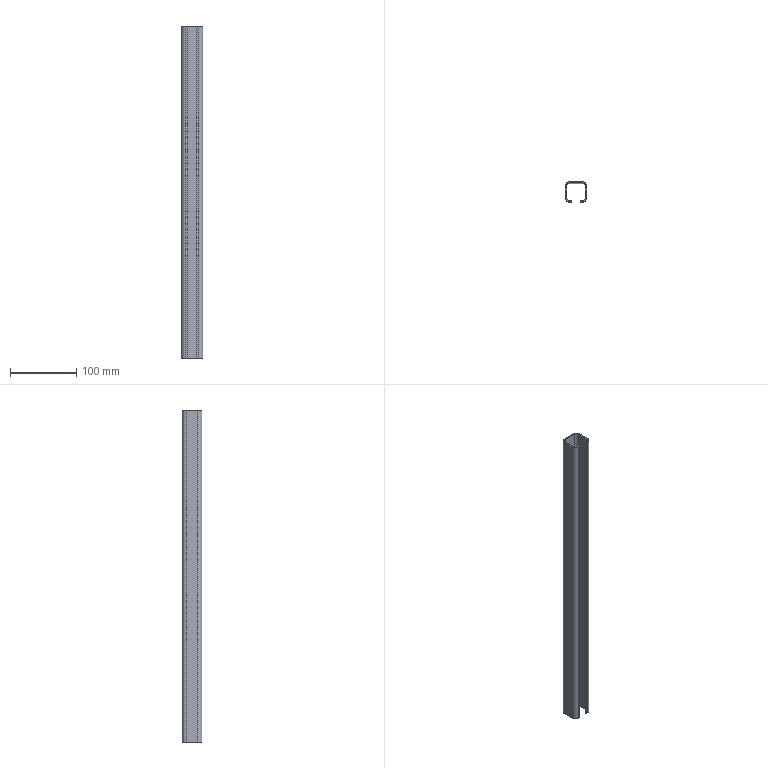Part | SolidWorks | features Extrusion 1 | 1 solid | 22 faces | box 32 x 30 x 500 mm | volume 85540 mm3 | plane 14 | cylinder 8 | commonest cylinder face diameters 8.4 x4 12 x4
STEP:
#1=CARTESIAN_POINT('',(-16.,-9.,0.));
#2=VERTEX_POINT('',#1);
#3=CARTESIAN_POINT('',(-10.,-15.,0.));
#4=VERTEX_POINT('',#3);
#5=CARTESIAN_POINT('',(-10.,-9.,0.));
#6=DIRECTION('',(0.,0.,1.));
#7=DIRECTION('',(1.,0.,0.));
#8=AXIS2_PLACEMENT_3D('',#5,#6,#7);
#9=CIRCLE('',#8,6.);
#10=EDGE_CURVE('',#2,#4,#9,.T.);
#11=ORIENTED_EDGE('',*,*,#10,.T.);
#12=CARTESIAN_POINT('',(-10.,-15.,500.));
#13=VERTEX_POINT('',#12);
#14=CARTESIAN_POINT('',(-10.,-15.,500.));
#15=DIRECTION('',(0.,0.,-1.));
#16=VECTOR('',#15,1000.);
#17=LINE('',#14,#16);
#18=EDGE_CURVE('',#13,#4,#17,.T.);
#19=ORIENTED_EDGE('',*,*,#18,.F.);
#20=CARTESIAN_POINT('',(-16.,-9.,500.));
#21=VERTEX_POINT('',#20);
#22=CARTESIAN_POINT('',(-10.,-9.,500.));
#23=DIRECTION('',(0.,0.,1.));
#24=DIRECTION('',(1.,0.,0.));
#25=AXIS2_PLACEMENT_3D('',#22,#23,#24);
#26=CIRCLE('',#25,6.);
#27=EDGE_CURVE('',#21,#13,#26,.T.);
#28=ORIENTED_EDGE('',*,*,#27,.F.);
#29=CARTESIAN_POINT('',(-16.,-9.,500.));
#30=DIRECTION('',(0.,0.,-1.));
#31=VECTOR('',#30,1000.);
#32=LINE('',#29,#31);
#33=EDGE_CURVE('',#21,#2,#32,.T.);
#34=ORIENTED_EDGE('',*,*,#33,.T.);
#35=EDGE_LOOP('',(#11,#19,#28,#34));
#36=FACE_OUTER_BOUND('',#35,.T.);
#37=CARTESIAN_POINT('',(-10.,-9.,500.));
#38=DIRECTION('',(0.,0.,-1.));
#39=DIRECTION('',(-1.,0.,0.));
#40=AXIS2_PLACEMENT_3D('',#37,#38,#39);
#41=CYLINDRICAL_SURFACE('',#40,6.);
#42=ADVANCED_FACE('',(#36),#41,.T.);
#43=CARTESIAN_POINT('',(-6.5,-15.,0.));
#44=VERTEX_POINT('',#43);
#45=CARTESIAN_POINT('',(-10.,-15.,0.));
#46=DIRECTION('',(1.,0.,0.));
#47=VECTOR('',#46,1000.);
#48=LINE('',#45,#47);
#49=EDGE_CURVE('',#4,#44,#48,.T.);
#50=ORIENTED_EDGE('',*,*,#49,.T.);
#51=CARTESIAN_POINT('',(-6.5,-15.,500.));
#52=VERTEX_POINT('',#51);
#53=CARTESIAN_POINT('',(-6.5,-15.,500.));
#54=DIRECTION('',(0.,0.,-1.));
#55=VECTOR('',#54,1000.);
#56=LINE('',#53,#55);
#57=EDGE_CURVE('',#52,#44,#56,.T.);
#58=ORIENTED_EDGE('',*,*,#57,.F.);
#59=CARTESIAN_POINT('',(-10.,-15.,500.));
#60=DIRECTION('',(1.,0.,0.));
#61=VECTOR('',#60,1000.);
#62=LINE('',#59,#61);
#63=EDGE_CURVE('',#13,#52,#62,.T.);
#64=ORIENTED_EDGE('',*,*,#63,.F.);
#65=ORIENTED_EDGE('',*,*,#18,.T.);
#66=EDGE_LOOP('',(#50,#58,#64,#65));
#67=FACE_OUTER_BOUND('',#66,.T.);
#68=CARTESIAN_POINT('',(-10.,-15.,500.));
#69=DIRECTION('',(0.,1.,0.));
#70=DIRECTION('',(-1.,0.,0.));
#71=AXIS2_PLACEMENT_3D('',#68,#69,#70);
#72=PLANE('',#71);
#73=ADVANCED_FACE('',(#67),#72,.F.);
#74=CARTESIAN_POINT('',(-6.5,-13.2,0.));
#75=VERTEX_POINT('',#74);
#76=CARTESIAN_POINT('',(-6.5,-15.,0.));
#77=DIRECTION('',(0.,1.,0.));
#78=VECTOR('',#77,1000.);
#79=LINE('',#76,#78);
#80=EDGE_CURVE('',#44,#75,#79,.T.);
#81=ORIENTED_EDGE('',*,*,#80,.T.);
#82=CARTESIAN_POINT('',(-6.5,-13.2,500.));
#83=VERTEX_POINT('',#82);
#84=CARTESIAN_POINT('',(-6.5,-13.2,500.));
#85=DIRECTION('',(0.,0.,-1.));
#86=VECTOR('',#85,1000.);
#87=LINE('',#84,#86);
#88=EDGE_CURVE('',#83,#75,#87,.T.);
#89=ORIENTED_EDGE('',*,*,#88,.F.);
#90=CARTESIAN_POINT('',(-6.5,-15.,500.));
#91=DIRECTION('',(0.,1.,0.));
#92=VECTOR('',#91,1000.);
#93=LINE('',#90,#92);
#94=EDGE_CURVE('',#52,#83,#93,.T.);
#95=ORIENTED_EDGE('',*,*,#94,.F.);
#96=ORIENTED_EDGE('',*,*,#57,.T.);
#97=EDGE_LOOP('',(#81,#89,#95,#96));
#98=FACE_OUTER_BOUND('',#97,.T.);
#99=CARTESIAN_POINT('',(-6.5,-15.,500.));
#100=DIRECTION('',(-1.,0.,0.));
#101=DIRECTION('',(0.,-1.,0.));
#102=AXIS2_PLACEMENT_3D('',#99,#100,#101);
#103=PLANE('',#102);
#104=ADVANCED_FACE('',(#98),#103,.F.);
#105=CARTESIAN_POINT('',(-10.,-13.2,0.));
#106=VERTEX_POINT('',#105);
#107=CARTESIAN_POINT('',(-10.,-13.2,0.));
#108=DIRECTION('',(-1.,0.,0.));
#109=VECTOR('',#108,1000.);
#110=LINE('',#107,#109);
#111=EDGE_CURVE('',#75,#106,#110,.T.);
#112=ORIENTED_EDGE('',*,*,#111,.T.);
#113=CARTESIAN_POINT('',(-10.,-13.2,500.));
#114=VERTEX_POINT('',#113);
#115=CARTESIAN_POINT('',(-10.,-13.2,500.));
#116=DIRECTION('',(0.,0.,-1.));
#117=VECTOR('',#116,1000.);
#118=LINE('',#115,#117);
#119=EDGE_CURVE('',#114,#106,#118,.T.);
#120=ORIENTED_EDGE('',*,*,#119,.F.);
#121=CARTESIAN_POINT('',(-10.,-13.2,500.));
#122=DIRECTION('',(-1.,0.,0.));
#123=VECTOR('',#122,1000.);
#124=LINE('',#121,#123);
#125=EDGE_CURVE('',#83,#114,#124,.T.);
#126=ORIENTED_EDGE('',*,*,#125,.F.);
#127=ORIENTED_EDGE('',*,*,#88,.T.);
#128=EDGE_LOOP('',(#112,#120,#126,#127));
#129=FACE_OUTER_BOUND('',#128,.T.);
#130=CARTESIAN_POINT('',(-10.,-13.2,500.));
#131=DIRECTION('',(0.,-1.,0.));
#132=DIRECTION('',(0.,0.,-1.));
#133=AXIS2_PLACEMENT_3D('',#130,#131,#132);
#134=PLANE('',#133);
#135=ADVANCED_FACE('',(#129),#134,.F.);
#136=CARTESIAN_POINT('',(-14.2,-9.,0.));
#137=VERTEX_POINT('',#136);
#138=CARTESIAN_POINT('',(-10.,-9.,0.));
#139=DIRECTION('',(0.,0.,-1.));
#140=DIRECTION('',(1.,0.,0.));
#141=AXIS2_PLACEMENT_3D('',#138,#139,#140);
#142=CIRCLE('',#141,4.2);
#143=EDGE_CURVE('',#106,#137,#142,.T.);
#144=ORIENTED_EDGE('',*,*,#143,.T.);
#145=CARTESIAN_POINT('',(-14.2,-9.,500.));
#146=VERTEX_POINT('',#145);
#147=CARTESIAN_POINT('',(-14.2,-9.,500.));
#148=DIRECTION('',(0.,0.,-1.));
#149=VECTOR('',#148,1000.);
#150=LINE('',#147,#149);
#151=EDGE_CURVE('',#146,#137,#150,.T.);
#152=ORIENTED_EDGE('',*,*,#151,.F.);
#153=CARTESIAN_POINT('',(-10.,-9.,500.));
#154=DIRECTION('',(0.,0.,-1.));
#155=DIRECTION('',(1.,0.,0.));
#156=AXIS2_PLACEMENT_3D('',#153,#154,#155);
#157=CIRCLE('',#156,4.2);
#158=EDGE_CURVE('',#114,#146,#157,.T.);
#159=ORIENTED_EDGE('',*,*,#158,.F.);
#160=ORIENTED_EDGE('',*,*,#119,.T.);
#161=EDGE_LOOP('',(#144,#152,#159,#160));
#162=FACE_OUTER_BOUND('',#161,.T.);
#163=CARTESIAN_POINT('',(-10.,-9.,500.));
#164=DIRECTION('',(0.,0.,-1.));
#165=DIRECTION('',(-1.,0.,0.));
#166=AXIS2_PLACEMENT_3D('',#163,#164,#165);
#167=CYLINDRICAL_SURFACE('',#166,4.2);
#168=ADVANCED_FACE('',(#162),#167,.F.);
#169=CARTESIAN_POINT('',(-14.2,9.,0.));
#170=VERTEX_POINT('',#169);
#171=CARTESIAN_POINT('',(-14.2,9.,0.));
#172=DIRECTION('',(0.,1.,0.));
#173=VECTOR('',#172,1000.);
#174=LINE('',#171,#173);
#175=EDGE_CURVE('',#137,#170,#174,.T.);
#176=ORIENTED_EDGE('',*,*,#175,.T.);
#177=CARTESIAN_POINT('',(-14.2,9.,500.));
#178=VERTEX_POINT('',#177);
#179=CARTESIAN_POINT('',(-14.2,9.,500.));
#180=DIRECTION('',(0.,0.,-1.));
#181=VECTOR('',#180,1000.);
#182=LINE('',#179,#181);
#183=EDGE_CURVE('',#178,#170,#182,.T.);
#184=ORIENTED_EDGE('',*,*,#183,.F.);
#185=CARTESIAN_POINT('',(-14.2,9.,500.));
#186=DIRECTION('',(0.,1.,0.));
#187=VECTOR('',#186,1000.);
#188=LINE('',#185,#187);
#189=EDGE_CURVE('',#146,#178,#188,.T.);
#190=ORIENTED_EDGE('',*,*,#189,.F.);
#191=ORIENTED_EDGE('',*,*,#151,.T.);
#192=EDGE_LOOP('',(#176,#184,#190,#191));
#193=FACE_OUTER_BOUND('',#192,.T.);
#194=CARTESIAN_POINT('',(-14.2,9.,500.));
#195=DIRECTION('',(-1.,0.,0.));
#196=DIRECTION('',(0.,0.,1.));
#197=AXIS2_PLACEMENT_3D('',#194,#195,#196);
#198=PLANE('',#197);
#199=ADVANCED_FACE('',(#193),#198,.F.);
#200=CARTESIAN_POINT('',(-10.,13.2,0.));
#201=VERTEX_POINT('',#200);
#202=CARTESIAN_POINT('',(-10.,9.,0.));
#203=DIRECTION('',(0.,0.,-1.));
#204=DIRECTION('',(1.,0.,0.));
#205=AXIS2_PLACEMENT_3D('',#202,#203,#204);
#206=CIRCLE('',#205,4.2);
#207=EDGE_CURVE('',#170,#201,#206,.T.);
#208=ORIENTED_EDGE('',*,*,#207,.T.);
#209=CARTESIAN_POINT('',(-10.,13.2,500.));
#210=VERTEX_POINT('',#209);
#211=CARTESIAN_POINT('',(-10.,13.2,500.));
#212=DIRECTION('',(0.,0.,-1.));
#213=VECTOR('',#212,1000.);
#214=LINE('',#211,#213);
#215=EDGE_CURVE('',#210,#201,#214,.T.);
#216=ORIENTED_EDGE('',*,*,#215,.F.);
#217=CARTESIAN_POINT('',(-10.,9.,500.));
#218=DIRECTION('',(0.,0.,-1.));
#219=DIRECTION('',(1.,0.,0.));
#220=AXIS2_PLACEMENT_3D('',#217,#218,#219);
#221=CIRCLE('',#220,4.2);
#222=EDGE_CURVE('',#178,#210,#221,.T.);
#223=ORIENTED_EDGE('',*,*,#222,.F.);
#224=ORIENTED_EDGE('',*,*,#183,.T.);
#225=EDGE_LOOP('',(#208,#216,#223,#224));
#226=FACE_OUTER_BOUND('',#225,.T.);
#227=CARTESIAN_POINT('',(-10.,9.,500.));
#228=DIRECTION('',(0.,0.,-1.));
#229=DIRECTION('',(-1.,0.,0.));
#230=AXIS2_PLACEMENT_3D('',#227,#228,#229);
#231=CYLINDRICAL_SURFACE('',#230,4.2);
#232=ADVANCED_FACE('',(#226),#231,.F.);
#233=CARTESIAN_POINT('',(10.,13.2,0.));
#234=VERTEX_POINT('',#233);
#235=CARTESIAN_POINT('',(-10.,13.2,0.));
#236=DIRECTION('',(1.,0.,0.));
#237=VECTOR('',#236,1000.);
#238=LINE('',#235,#237);
#239=EDGE_CURVE('',#201,#234,#238,.T.);
#240=ORIENTED_EDGE('',*,*,#239,.T.);
#241=CARTESIAN_POINT('',(10.,13.2,500.));
#242=VERTEX_POINT('',#241);
#243=CARTESIAN_POINT('',(10.,13.2,500.));
#244=DIRECTION('',(0.,0.,-1.));
#245=VECTOR('',#244,1000.);
#246=LINE('',#243,#245);
#247=EDGE_CURVE('',#242,#234,#246,.T.);
#248=ORIENTED_EDGE('',*,*,#247,.F.);
#249=CARTESIAN_POINT('',(-10.,13.2,500.));
#250=DIRECTION('',(1.,0.,0.));
#251=VECTOR('',#250,1000.);
#252=LINE('',#249,#251);
#253=EDGE_CURVE('',#210,#242,#252,.T.);
#254=ORIENTED_EDGE('',*,*,#253,.F.);
#255=ORIENTED_EDGE('',*,*,#215,.T.);
#256=EDGE_LOOP('',(#240,#248,#254,#255));
#257=FACE_OUTER_BOUND('',#256,.T.);
#258=CARTESIAN_POINT('',(-10.,13.2,500.));
#259=DIRECTION('',(0.,1.,0.));
#260=DIRECTION('',(-1.,0.,0.));
#261=AXIS2_PLACEMENT_3D('',#258,#259,#260);
#262=PLANE('',#261);
#263=ADVANCED_FACE('',(#257),#262,.F.);
#264=CARTESIAN_POINT('',(14.2,9.,0.));
#265=VERTEX_POINT('',#264);
#266=CARTESIAN_POINT('',(10.,9.,0.));
#267=DIRECTION('',(0.,0.,-1.));
#268=DIRECTION('',(-1.,0.,0.));
#269=AXIS2_PLACEMENT_3D('',#266,#267,#268);
#270=CIRCLE('',#269,4.2);
#271=EDGE_CURVE('',#234,#265,#270,.T.);
#272=ORIENTED_EDGE('',*,*,#271,.T.);
#273=CARTESIAN_POINT('',(14.2,9.,500.));
#274=VERTEX_POINT('',#273);
#275=CARTESIAN_POINT('',(14.2,9.,500.));
#276=DIRECTION('',(0.,0.,-1.));
#277=VECTOR('',#276,1000.);
#278=LINE('',#275,#277);
#279=EDGE_CURVE('',#274,#265,#278,.T.);
#280=ORIENTED_EDGE('',*,*,#279,.F.);
#281=CARTESIAN_POINT('',(10.,9.,500.));
#282=DIRECTION('',(0.,0.,-1.));
#283=DIRECTION('',(-1.,0.,0.));
#284=AXIS2_PLACEMENT_3D('',#281,#282,#283);
#285=CIRCLE('',#284,4.2);
#286=EDGE_CURVE('',#242,#274,#285,.T.);
#287=ORIENTED_EDGE('',*,*,#286,.F.);
#288=ORIENTED_EDGE('',*,*,#247,.T.);
#289=EDGE_LOOP('',(#272,#280,#287,#288));
#290=FACE_OUTER_BOUND('',#289,.T.);
#291=CARTESIAN_POINT('',(10.,9.,500.));
#292=DIRECTION('',(0.,0.,-1.));
#293=DIRECTION('',(-1.,0.,0.));
#294=AXIS2_PLACEMENT_3D('',#291,#292,#293);
#295=CYLINDRICAL_SURFACE('',#294,4.2);
#296=ADVANCED_FACE('',(#290),#295,.F.);
#297=CARTESIAN_POINT('',(14.2,-9.,0.));
#298=VERTEX_POINT('',#297);
#299=CARTESIAN_POINT('',(14.2,9.,0.));
#300=DIRECTION('',(0.,-1.,0.));
#301=VECTOR('',#300,1000.);
#302=LINE('',#299,#301);
#303=EDGE_CURVE('',#265,#298,#302,.T.);
#304=ORIENTED_EDGE('',*,*,#303,.T.);
#305=CARTESIAN_POINT('',(14.2,-9.,500.));
#306=VERTEX_POINT('',#305);
#307=CARTESIAN_POINT('',(14.2,-9.,500.));
#308=DIRECTION('',(0.,0.,-1.));
#309=VECTOR('',#308,1000.);
#310=LINE('',#307,#309);
#311=EDGE_CURVE('',#306,#298,#310,.T.);
#312=ORIENTED_EDGE('',*,*,#311,.F.);
#313=CARTESIAN_POINT('',(14.2,9.,500.));
#314=DIRECTION('',(0.,-1.,0.));
#315=VECTOR('',#314,1000.);
#316=LINE('',#313,#315);
#317=EDGE_CURVE('',#274,#306,#316,.T.);
#318=ORIENTED_EDGE('',*,*,#317,.F.);
#319=ORIENTED_EDGE('',*,*,#279,.T.);
#320=EDGE_LOOP('',(#304,#312,#318,#319));
#321=FACE_OUTER_BOUND('',#320,.T.);
#322=CARTESIAN_POINT('',(14.2,9.,500.));
#323=DIRECTION('',(1.,0.,0.));
#324=DIRECTION('',(0.,1.,0.));
#325=AXIS2_PLACEMENT_3D('',#322,#323,#324);
#326=PLANE('',#325);
#327=ADVANCED_FACE('',(#321),#326,.F.);
#328=CARTESIAN_POINT('',(10.,-13.2,0.));
#329=VERTEX_POINT('',#328);
#330=CARTESIAN_POINT('',(10.,-9.,0.));
#331=DIRECTION('',(0.,0.,-1.));
#332=DIRECTION('',(1.,0.,0.));
#333=AXIS2_PLACEMENT_3D('',#330,#331,#332);
#334=CIRCLE('',#333,4.2);
#335=EDGE_CURVE('',#298,#329,#334,.T.);
#336=ORIENTED_EDGE('',*,*,#335,.T.);
#337=CARTESIAN_POINT('',(10.,-13.2,500.));
#338=VERTEX_POINT('',#337);
#339=CARTESIAN_POINT('',(10.,-13.2,500.));
#340=DIRECTION('',(0.,0.,-1.));
#341=VECTOR('',#340,1000.);
#342=LINE('',#339,#341);
#343=EDGE_CURVE('',#338,#329,#342,.T.);
#344=ORIENTED_EDGE('',*,*,#343,.F.);
#345=CARTESIAN_POINT('',(10.,-9.,500.));
#346=DIRECTION('',(0.,0.,-1.));
#347=DIRECTION('',(1.,0.,0.));
#348=AXIS2_PLACEMENT_3D('',#345,#346,#347);
#349=CIRCLE('',#348,4.2);
#350=EDGE_CURVE('',#306,#338,#349,.T.);
#351=ORIENTED_EDGE('',*,*,#350,.F.);
#352=ORIENTED_EDGE('',*,*,#311,.T.);
#353=EDGE_LOOP('',(#336,#344,#351,#352));
#354=FACE_OUTER_BOUND('',#353,.T.);
#355=CARTESIAN_POINT('',(10.,-9.,500.));
#356=DIRECTION('',(0.,0.,-1.));
#357=DIRECTION('',(-1.,0.,0.));
#358=AXIS2_PLACEMENT_3D('',#355,#356,#357);
#359=CYLINDRICAL_SURFACE('',#358,4.2);
#360=ADVANCED_FACE('',(#354),#359,.F.);
#361=CARTESIAN_POINT('',(6.5,-13.2,0.));
#362=VERTEX_POINT('',#361);
#363=CARTESIAN_POINT('',(6.5,-13.2,0.));
#364=DIRECTION('',(-1.,0.,0.));
#365=VECTOR('',#364,1000.);
#366=LINE('',#363,#365);
#367=EDGE_CURVE('',#329,#362,#366,.T.);
#368=ORIENTED_EDGE('',*,*,#367,.T.);
#369=CARTESIAN_POINT('',(6.5,-13.2,500.));
#370=VERTEX_POINT('',#369);
#371=CARTESIAN_POINT('',(6.5,-13.2,500.));
#372=DIRECTION('',(0.,0.,-1.));
#373=VECTOR('',#372,1000.);
#374=LINE('',#371,#373);
#375=EDGE_CURVE('',#370,#362,#374,.T.);
#376=ORIENTED_EDGE('',*,*,#375,.F.);
#377=CARTESIAN_POINT('',(6.5,-13.2,500.));
#378=DIRECTION('',(-1.,0.,0.));
#379=VECTOR('',#378,1000.);
#380=LINE('',#377,#379);
#381=EDGE_CURVE('',#338,#370,#380,.T.);
#382=ORIENTED_EDGE('',*,*,#381,.F.);
#383=ORIENTED_EDGE('',*,*,#343,.T.);
#384=EDGE_LOOP('',(#368,#376,#382,#383));
#385=FACE_OUTER_BOUND('',#384,.T.);
#386=CARTESIAN_POINT('',(6.5,-13.2,500.));
#387=DIRECTION('',(0.,-1.,0.));
#388=DIRECTION('',(1.,0.,0.));
#389=AXIS2_PLACEMENT_3D('',#386,#387,#388);
#390=PLANE('',#389);
#391=ADVANCED_FACE('',(#385),#390,.F.);
#392=CARTESIAN_POINT('',(6.5,-15.,0.));
#393=VERTEX_POINT('',#392);
#394=CARTESIAN_POINT('',(6.5,-15.,0.));
#395=DIRECTION('',(0.,-1.,0.));
#396=VECTOR('',#395,1000.);
#397=LINE('',#394,#396);
#398=EDGE_CURVE('',#362,#393,#397,.T.);
#399=ORIENTED_EDGE('',*,*,#398,.T.);
#400=CARTESIAN_POINT('',(6.5,-15.,500.));
#401=VERTEX_POINT('',#400);
#402=CARTESIAN_POINT('',(6.5,-15.,500.));
#403=DIRECTION('',(0.,0.,-1.));
#404=VECTOR('',#403,1000.);
#405=LINE('',#402,#404);
#406=EDGE_CURVE('',#401,#393,#405,.T.);
#407=ORIENTED_EDGE('',*,*,#406,.F.);
#408=CARTESIAN_POINT('',(6.5,-15.,500.));
#409=DIRECTION('',(0.,-1.,0.));
#410=VECTOR('',#409,1000.);
#411=LINE('',#408,#410);
#412=EDGE_CURVE('',#370,#401,#411,.T.);
#413=ORIENTED_EDGE('',*,*,#412,.F.);
#414=ORIENTED_EDGE('',*,*,#375,.T.);
#415=EDGE_LOOP('',(#399,#407,#413,#414));
#416=FACE_OUTER_BOUND('',#415,.T.);
#417=CARTESIAN_POINT('',(6.5,-15.,500.));
#418=DIRECTION('',(1.,0.,0.));
#419=DIRECTION('',(0.,1.,0.));
#420=AXIS2_PLACEMENT_3D('',#417,#418,#419);
#421=PLANE('',#420);
#422=ADVANCED_FACE('',(#416),#421,.F.);
#423=CARTESIAN_POINT('',(10.,-15.,0.));
#424=VERTEX_POINT('',#423);
#425=CARTESIAN_POINT('',(6.5,-15.,0.));
#426=DIRECTION('',(1.,0.,0.));
#427=VECTOR('',#426,1000.);
#428=LINE('',#425,#427);
#429=EDGE_CURVE('',#393,#424,#428,.T.);
#430=ORIENTED_EDGE('',*,*,#429,.T.);
#431=CARTESIAN_POINT('',(10.,-15.,500.));
#432=VERTEX_POINT('',#431);
#433=CARTESIAN_POINT('',(10.,-15.,500.));
#434=DIRECTION('',(0.,0.,-1.));
#435=VECTOR('',#434,1000.);
#436=LINE('',#433,#435);
#437=EDGE_CURVE('',#432,#424,#436,.T.);
#438=ORIENTED_EDGE('',*,*,#437,.F.);
#439=CARTESIAN_POINT('',(6.5,-15.,500.));
#440=DIRECTION('',(1.,0.,0.));
#441=VECTOR('',#440,1000.);
#442=LINE('',#439,#441);
#443=EDGE_CURVE('',#401,#432,#442,.T.);
#444=ORIENTED_EDGE('',*,*,#443,.F.);
#445=ORIENTED_EDGE('',*,*,#406,.T.);
#446=EDGE_LOOP('',(#430,#438,#444,#445));
#447=FACE_OUTER_BOUND('',#446,.T.);
#448=CARTESIAN_POINT('',(6.5,-15.,500.));
#449=DIRECTION('',(0.,1.,0.));
#450=DIRECTION('',(0.,0.,1.));
#451=AXIS2_PLACEMENT_3D('',#448,#449,#450);
#452=PLANE('',#451);
#453=ADVANCED_FACE('',(#447),#452,.F.);
#454=CARTESIAN_POINT('',(16.,-9.,0.));
#455=VERTEX_POINT('',#454);
#456=CARTESIAN_POINT('',(10.,-9.,0.));
#457=DIRECTION('',(0.,0.,1.));
#458=DIRECTION('',(1.,0.,0.));
#459=AXIS2_PLACEMENT_3D('',#456,#457,#458);
#460=CIRCLE('',#459,6.);
#461=EDGE_CURVE('',#424,#455,#460,.T.);
#462=ORIENTED_EDGE('',*,*,#461,.T.);
#463=CARTESIAN_POINT('',(16.,-9.,500.));
#464=VERTEX_POINT('',#463);
#465=CARTESIAN_POINT('',(16.,-9.,500.));
#466=DIRECTION('',(0.,0.,-1.));
#467=VECTOR('',#466,1000.);
#468=LINE('',#465,#467);
#469=EDGE_CURVE('',#464,#455,#468,.T.);
#470=ORIENTED_EDGE('',*,*,#469,.F.);
#471=CARTESIAN_POINT('',(10.,-9.,500.));
#472=DIRECTION('',(0.,0.,1.));
#473=DIRECTION('',(1.,0.,0.));
#474=AXIS2_PLACEMENT_3D('',#471,#472,#473);
#475=CIRCLE('',#474,6.);
#476=EDGE_CURVE('',#432,#464,#475,.T.);
#477=ORIENTED_EDGE('',*,*,#476,.F.);
#478=ORIENTED_EDGE('',*,*,#437,.T.);
#479=EDGE_LOOP('',(#462,#470,#477,#478));
#480=FACE_OUTER_BOUND('',#479,.T.);
#481=CARTESIAN_POINT('',(10.,-9.,500.));
#482=DIRECTION('',(0.,0.,-1.));
#483=DIRECTION('',(-1.,0.,0.));
#484=AXIS2_PLACEMENT_3D('',#481,#482,#483);
#485=CYLINDRICAL_SURFACE('',#484,6.);
#486=ADVANCED_FACE('',(#480),#485,.T.);
#487=CARTESIAN_POINT('',(16.,9.,0.));
#488=VERTEX_POINT('',#487);
#489=CARTESIAN_POINT('',(16.,9.,0.));
#490=DIRECTION('',(0.,1.,0.));
#491=VECTOR('',#490,1000.);
#492=LINE('',#489,#491);
#493=EDGE_CURVE('',#455,#488,#492,.T.);
#494=ORIENTED_EDGE('',*,*,#493,.T.);
#495=CARTESIAN_POINT('',(16.,9.,500.));
#496=VERTEX_POINT('',#495);
#497=CARTESIAN_POINT('',(16.,9.,500.));
#498=DIRECTION('',(0.,0.,-1.));
#499=VECTOR('',#498,1000.);
#500=LINE('',#497,#499);
#501=EDGE_CURVE('',#496,#488,#500,.T.);
#502=ORIENTED_EDGE('',*,*,#501,.F.);
#503=CARTESIAN_POINT('',(16.,9.,500.));
#504=DIRECTION('',(0.,1.,0.));
#505=VECTOR('',#504,1000.);
#506=LINE('',#503,#505);
#507=EDGE_CURVE('',#464,#496,#506,.T.);
#508=ORIENTED_EDGE('',*,*,#507,.F.);
#509=ORIENTED_EDGE('',*,*,#469,.T.);
#510=EDGE_LOOP('',(#494,#502,#508,#509));
#511=FACE_OUTER_BOUND('',#510,.T.);
#512=CARTESIAN_POINT('',(16.,9.,500.));
#513=DIRECTION('',(-1.,0.,0.));
#514=DIRECTION('',(0.,-1.,0.));
#515=AXIS2_PLACEMENT_3D('',#512,#513,#514);
#516=PLANE('',#515);
#517=ADVANCED_FACE('',(#511),#516,.F.);
#518=CARTESIAN_POINT('',(10.,15.,0.));
#519=VERTEX_POINT('',#518);
#520=CARTESIAN_POINT('',(10.,9.,0.));
#521=DIRECTION('',(0.,0.,1.));
#522=DIRECTION('',(-1.,0.,0.));
#523=AXIS2_PLACEMENT_3D('',#520,#521,#522);
#524=CIRCLE('',#523,6.);
#525=EDGE_CURVE('',#488,#519,#524,.T.);
#526=ORIENTED_EDGE('',*,*,#525,.T.);
#527=CARTESIAN_POINT('',(10.,15.,500.));
#528=VERTEX_POINT('',#527);
#529=CARTESIAN_POINT('',(10.,15.,500.));
#530=DIRECTION('',(0.,0.,-1.));
#531=VECTOR('',#530,1000.);
#532=LINE('',#529,#531);
#533=EDGE_CURVE('',#528,#519,#532,.T.);
#534=ORIENTED_EDGE('',*,*,#533,.F.);
#535=CARTESIAN_POINT('',(10.,9.,500.));
#536=DIRECTION('',(0.,0.,1.));
#537=DIRECTION('',(-1.,0.,0.));
#538=AXIS2_PLACEMENT_3D('',#535,#536,#537);
#539=CIRCLE('',#538,6.);
#540=EDGE_CURVE('',#496,#528,#539,.T.);
#541=ORIENTED_EDGE('',*,*,#540,.F.);
#542=ORIENTED_EDGE('',*,*,#501,.T.);
#543=EDGE_LOOP('',(#526,#534,#541,#542));
#544=FACE_OUTER_BOUND('',#543,.T.);
#545=CARTESIAN_POINT('',(10.,9.,500.));
#546=DIRECTION('',(0.,0.,-1.));
#547=DIRECTION('',(-1.,0.,0.));
#548=AXIS2_PLACEMENT_3D('',#545,#546,#547);
#549=CYLINDRICAL_SURFACE('',#548,6.);
#550=ADVANCED_FACE('',(#544),#549,.T.);
#551=CARTESIAN_POINT('',(-10.,15.,0.));
#552=VERTEX_POINT('',#551);
#553=CARTESIAN_POINT('',(-10.,15.,0.));
#554=DIRECTION('',(-1.,0.,0.));
#555=VECTOR('',#554,1000.);
#556=LINE('',#553,#555);
#557=EDGE_CURVE('',#519,#552,#556,.T.);
#558=ORIENTED_EDGE('',*,*,#557,.T.);
#559=CARTESIAN_POINT('',(-10.,15.,500.));
#560=VERTEX_POINT('',#559);
#561=CARTESIAN_POINT('',(-10.,15.,500.));
#562=DIRECTION('',(0.,0.,-1.));
#563=VECTOR('',#562,1000.);
#564=LINE('',#561,#563);
#565=EDGE_CURVE('',#560,#552,#564,.T.);
#566=ORIENTED_EDGE('',*,*,#565,.F.);
#567=CARTESIAN_POINT('',(-10.,15.,500.));
#568=DIRECTION('',(-1.,0.,0.));
#569=VECTOR('',#568,1000.);
#570=LINE('',#567,#569);
#571=EDGE_CURVE('',#528,#560,#570,.T.);
#572=ORIENTED_EDGE('',*,*,#571,.F.);
#573=ORIENTED_EDGE('',*,*,#533,.T.);
#574=EDGE_LOOP('',(#558,#566,#572,#573));
#575=FACE_OUTER_BOUND('',#574,.T.);
#576=CARTESIAN_POINT('',(-10.,15.,500.));
#577=DIRECTION('',(0.,-1.,0.));
#578=DIRECTION('',(0.,0.,-1.));
#579=AXIS2_PLACEMENT_3D('',#576,#577,#578);
#580=PLANE('',#579);
#581=ADVANCED_FACE('',(#575),#580,.F.);
#582=CARTESIAN_POINT('',(-16.,9.,0.));
#583=VERTEX_POINT('',#582);
#584=CARTESIAN_POINT('',(-10.,9.,0.));
#585=DIRECTION('',(0.,0.,1.));
#586=DIRECTION('',(1.,0.,0.));
#587=AXIS2_PLACEMENT_3D('',#584,#585,#586);
#588=CIRCLE('',#587,6.);
#589=EDGE_CURVE('',#552,#583,#588,.T.);
#590=ORIENTED_EDGE('',*,*,#589,.T.);
#591=CARTESIAN_POINT('',(-16.,9.,500.));
#592=VERTEX_POINT('',#591);
#593=CARTESIAN_POINT('',(-16.,9.,500.));
#594=DIRECTION('',(0.,0.,-1.));
#595=VECTOR('',#594,1000.);
#596=LINE('',#593,#595);
#597=EDGE_CURVE('',#592,#583,#596,.T.);
#598=ORIENTED_EDGE('',*,*,#597,.F.);
#599=CARTESIAN_POINT('',(-10.,9.,500.));
#600=DIRECTION('',(0.,0.,1.));
#601=DIRECTION('',(1.,0.,0.));
#602=AXIS2_PLACEMENT_3D('',#599,#600,#601);
#603=CIRCLE('',#602,6.);
#604=EDGE_CURVE('',#560,#592,#603,.T.);
#605=ORIENTED_EDGE('',*,*,#604,.F.);
#606=ORIENTED_EDGE('',*,*,#565,.T.);
#607=EDGE_LOOP('',(#590,#598,#605,#606));
#608=FACE_OUTER_BOUND('',#607,.T.);
#609=CARTESIAN_POINT('',(-10.,9.,500.));
#610=DIRECTION('',(0.,0.,-1.));
#611=DIRECTION('',(-1.,0.,0.));
#612=AXIS2_PLACEMENT_3D('',#609,#610,#611);
#613=CYLINDRICAL_SURFACE('',#612,6.);
#614=ADVANCED_FACE('',(#608),#613,.T.);
#615=CARTESIAN_POINT('',(-16.,9.,0.));
#616=DIRECTION('',(0.,-1.,0.));
#617=VECTOR('',#616,1000.);
#618=LINE('',#615,#617);
#619=EDGE_CURVE('',#583,#2,#618,.T.);
#620=ORIENTED_EDGE('',*,*,#619,.T.);
#621=ORIENTED_EDGE('',*,*,#33,.F.);
#622=CARTESIAN_POINT('',(-16.,9.,500.));
#623=DIRECTION('',(0.,-1.,0.));
#624=VECTOR('',#623,1000.);
#625=LINE('',#622,#624);
#626=EDGE_CURVE('',#592,#21,#625,.T.);
#627=ORIENTED_EDGE('',*,*,#626,.F.);
#628=ORIENTED_EDGE('',*,*,#597,.T.);
#629=EDGE_LOOP('',(#620,#621,#627,#628));
#630=FACE_OUTER_BOUND('',#629,.T.);
#631=CARTESIAN_POINT('',(-16.,9.,500.));
#632=DIRECTION('',(1.,0.,0.));
#633=DIRECTION('',(0.,0.,-1.));
#634=AXIS2_PLACEMENT_3D('',#631,#632,#633);
#635=PLANE('',#634);
#636=ADVANCED_FACE('',(#630),#635,.F.);
#637=ORIENTED_EDGE('',*,*,#27,.T.);
#638=ORIENTED_EDGE('',*,*,#63,.T.);
#639=ORIENTED_EDGE('',*,*,#94,.T.);
#640=ORIENTED_EDGE('',*,*,#125,.T.);
#641=ORIENTED_EDGE('',*,*,#158,.T.);
#642=ORIENTED_EDGE('',*,*,#189,.T.);
#643=ORIENTED_EDGE('',*,*,#222,.T.);
#644=ORIENTED_EDGE('',*,*,#253,.T.);
#645=ORIENTED_EDGE('',*,*,#286,.T.);
#646=ORIENTED_EDGE('',*,*,#317,.T.);
#647=ORIENTED_EDGE('',*,*,#350,.T.);
#648=ORIENTED_EDGE('',*,*,#381,.T.);
#649=ORIENTED_EDGE('',*,*,#412,.T.);
#650=ORIENTED_EDGE('',*,*,#443,.T.);
#651=ORIENTED_EDGE('',*,*,#476,.T.);
#652=ORIENTED_EDGE('',*,*,#507,.T.);
#653=ORIENTED_EDGE('',*,*,#540,.T.);
#654=ORIENTED_EDGE('',*,*,#571,.T.);
#655=ORIENTED_EDGE('',*,*,#604,.T.);
#656=ORIENTED_EDGE('',*,*,#626,.T.);
#657=EDGE_LOOP('',(#637,#638,#639,#640,#641,#642,#643,#644,#645,#646,#647,#648,#649,#650,#651,#652,#653,#654,#655,#656));
#658=FACE_OUTER_BOUND('',#657,.T.);
#659=CARTESIAN_POINT('',(-10.,-9.,500.));
#660=DIRECTION('',(0.,0.,1.));
#661=DIRECTION('',(1.,0.,0.));
#662=AXIS2_PLACEMENT_3D('',#659,#660,#661);
#663=PLANE('',#662);
#664=ADVANCED_FACE('',(#658),#663,.T.);
#665=ORIENTED_EDGE('',*,*,#10,.F.);
#666=ORIENTED_EDGE('',*,*,#619,.F.);
#667=ORIENTED_EDGE('',*,*,#589,.F.);
#668=ORIENTED_EDGE('',*,*,#557,.F.);
#669=ORIENTED_EDGE('',*,*,#525,.F.);
#670=ORIENTED_EDGE('',*,*,#493,.F.);
#671=ORIENTED_EDGE('',*,*,#461,.F.);
#672=ORIENTED_EDGE('',*,*,#429,.F.);
#673=ORIENTED_EDGE('',*,*,#398,.F.);
#674=ORIENTED_EDGE('',*,*,#367,.F.);
#675=ORIENTED_EDGE('',*,*,#335,.F.);
#676=ORIENTED_EDGE('',*,*,#303,.F.);
#677=ORIENTED_EDGE('',*,*,#271,.F.);
#678=ORIENTED_EDGE('',*,*,#239,.F.);
#679=ORIENTED_EDGE('',*,*,#207,.F.);
#680=ORIENTED_EDGE('',*,*,#175,.F.);
#681=ORIENTED_EDGE('',*,*,#143,.F.);
#682=ORIENTED_EDGE('',*,*,#111,.F.);
#683=ORIENTED_EDGE('',*,*,#80,.F.);
#684=ORIENTED_EDGE('',*,*,#49,.F.);
#685=EDGE_LOOP('',(#665,#666,#667,#668,#669,#670,#671,#672,#673,#674,#675,#676,#677,#678,#679,#680,#681,#682,#683,#684));
#686=FACE_OUTER_BOUND('',#685,.T.);
#687=CARTESIAN_POINT('',(-10.,-9.,0.));
#688=DIRECTION('',(0.,0.,1.));
#689=DIRECTION('',(1.,0.,0.));
#690=AXIS2_PLACEMENT_3D('',#687,#688,#689);
#691=PLANE('',#690);
#692=ADVANCED_FACE('',(#686),#691,.F.);
#693=CLOSED_SHELL('',(#42,#73,#104,#135,#168,#199,#232,#263,#296,#327,#360,#391,#422,#453,#486,#517,#550,#581,#614,#636,#664,#692));
#694=MANIFOLD_SOLID_BREP('',#693);
#695=CARTESIAN_POINT('',(0.,0.,0.));
#696=DIRECTION('',(0.,0.,1.));
#697=DIRECTION('',(1.,0.,0.));
#698=AXIS2_PLACEMENT_3D('',#695,#696,#697);
#699=(LENGTH_UNIT()NAMED_UNIT(*)SI_UNIT(.MILLI.,.METRE.));
#700=UNCERTAINTY_MEASURE_WITH_UNIT(LENGTH_MEASURE(0.00001),#699,'','');
#701=(NAMED_UNIT(*)PLANE_ANGLE_UNIT()SI_UNIT($,.RADIAN.));
#702=(NAMED_UNIT(*)SI_UNIT($,.STERADIAN.)SOLID_ANGLE_UNIT());
#703=(GEOMETRIC_REPRESENTATION_CONTEXT(3)GLOBAL_UNCERTAINTY_ASSIGNED_CONTEXT((#700))GLOBAL_UNIT_ASSIGNED_CONTEXT((#699,#701,#702))REPRESENTATION_CONTEXT('',''));
#704=ADVANCED_BREP_SHAPE_REPRESENTATION('',(#694,#698),#703);